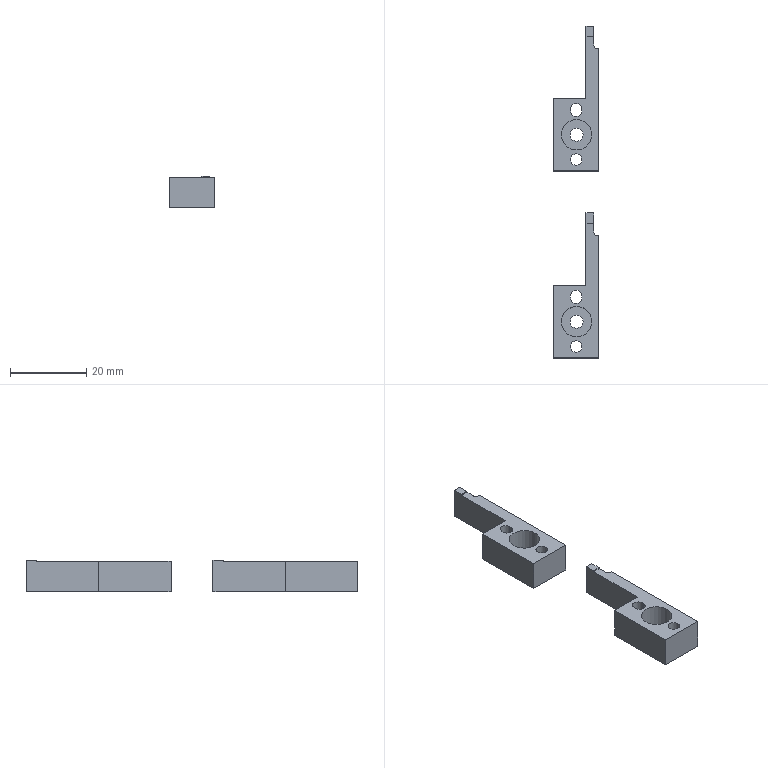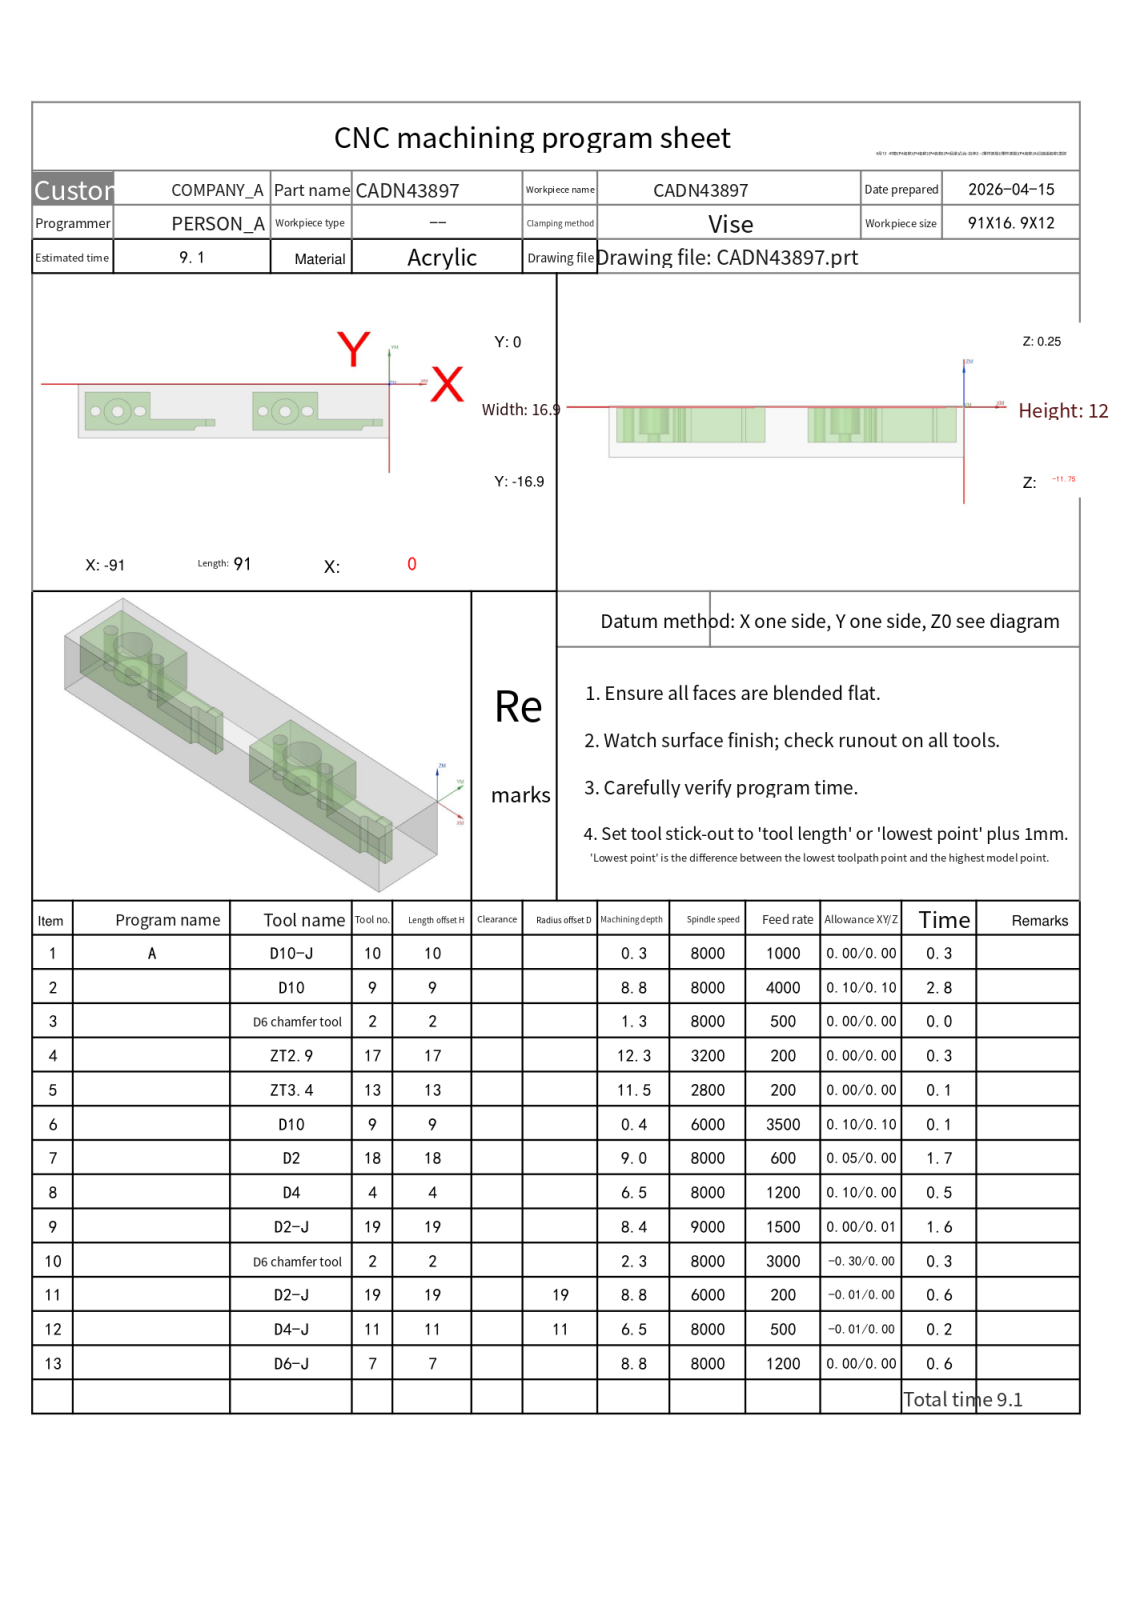NC program | NX | posted by the shop | part box 11.9 x 87 x 8.25 mm
Lines 8226 to 9110 of 9110:
N10 T02 M06
(D6 chamfer tool  D=6. R=0. H=02 ce=0.00 di=0.00)
G00 G90 G54 X-5.398 Y-9.389 M03 S8000
G43 H02 Z20.
M08
Z2.435
G01 Z-1.5 F3000.
X-5.404 Y-9.456
G03 X-5.111 Y-9.81 I.36 J0.0
G01 X-5.092 Y-9.809
X-4.989 Y-9.773
X-4.7 Y-9.74
X-3.35
X-2.
G02 X-.7 Y-11.04 I0.0 J-1.3
G01 Y-13.1
G02 X-2. Y-14.4 I-1.3 J0.0
G01 X-4.7
X-4.989 Y-14.367
X-5.092 Y-14.331
X-5.111 Y-14.33
G03 X-5.404 Y-14.684 I.067 J-.354
G01 X-5.398 Y-14.751
Z2.435
G00 Z20.
X-54.398 Y-9.389
Z2.435
G01 Z-1.5
X-54.404 Y-9.456
G03 X-54.111 Y-9.81 I.36 J0.0
G01 X-54.092 Y-9.809
X-53.989 Y-9.773
X-53.7 Y-9.74
X-51.
G02 X-49.7 Y-11.04 I0.0 J-1.3
G01 Y-12.07
Y-13.1
G02 X-51. Y-14.4 I-1.3 J0.0
G01 X-53.7
X-53.989 Y-14.367
X-54.092 Y-14.331
X-54.111 Y-14.33
G03 X-54.404 Y-14.684 I.067 J-.354
G01 X-54.398 Y-14.751
Z2.435
G00 Z6.
X-54.806 Y-14.566
Z2.512
G01 Z-1.75
X-54.78 Y-14.506
X-54.798 Y-14.441
X-54.85 Y-14.402
X-54.856 Y-14.4
X-55.7
G02 X-57. Y-15.7 I-1.3 J0.0
G01 X-60.
X-62.
X-63.
X-66.
X-67.
X-69.
X-74.
X-75.
X-77.
X-80.
X-81.
X-84.
X-86.
X-87.
X-89.
G02 X-90.3 Y-14.4 I0.0 J1.3
G01 Y-12.913
Y-11.425
Y-8.45
Y-2.5
G02 X-89. Y-1.2 I1.3 J0.0
G01 X-87.813
X-86.625
X-84.25
X-80.688
X-79.5
X-75.938
X-73.563
X-72.375
X-70.
G02 X-68.7 Y-2.5 I0.0 J-1.3
G01 Y-3.405
Y-4.31
Y-6.12
Y-9.74
X-67.763
X-66.825
X-64.95
X-62.138
X-61.2
X-58.388
X-56.513
X-55.575
X-54.843
Z2.677
G00 Z20.
X-73.125 Y-8.286
Z2.691
G01 Z-1.75
X-73.165 Y-8.436
G03 X-73.015 Y-8.696 I.3 J0.0
G01 X-73. Y-8.7
X-72.75
X-72.65 Y-8.673
X-72.577 Y-8.6
X-72.55 Y-8.5
X-72.577 Y-8.4
X-72.65 Y-8.327
X-72.75 Y-8.3
X-73.25
X-73.35 Y-8.327
X-73.423 Y-8.4
X-73.45 Y-8.5
X-73.423 Y-8.6
X-73.35 Y-8.673
X-73.25 Y-8.7
X-73.
X-72.985 Y-8.696
G03 X-72.835 Y-8.436 I-.15 J.26
G01 X-72.875 Y-8.286
Z2.691
G00 Z20.
X-5.806 Y-14.566
Z2.512
G01 Z-1.75
X-5.78 Y-14.506
X-5.798 Y-14.441
X-5.85 Y-14.402
X-5.856 Y-14.4
X-6.7
G02 X-8. Y-15.7 I-1.3 J0.0
G01 X-9.
X-10.
X-11.
X-12.
X-13.
X-14.
X-15.
X-16.
X-17.
X-18.
X-19.
X-20.
X-21.
X-22.
X-24.
X-25.
X-26.
X-27.
X-28.
X-29.
X-30.
X-31.
X-32.
X-33.
X-34.
X-35.
X-36.
X-37.
X-38.
X-40.
G02 X-41.3 Y-14.4 I0.0 J1.3
G01 Y-12.913
Y-11.425
Y-9.938
Y-8.45
Y-6.963
Y-5.475
Y-2.5
G02 X-40. Y-1.2 I1.3 J0.0
G01 X-38.813
X-37.625
X-36.438
X-35.25
X-34.063
X-32.875
X-31.688
X-30.5
X-29.313
X-28.125
X-26.938
X-25.75
X-24.563
X-23.375
X-21.
G02 X-19.7 Y-2.5 I0.0 J-1.3
G01 Y-3.405
Y-4.31
Y-5.215
Y-6.12
Y-7.025
Y-7.93
Y-9.74
X-18.763
X-17.825
X-16.888
X-15.95
X-15.013
X-14.075
X-13.138
X-12.2
X-11.263
X-10.325
X-9.388
X-8.45
X-7.513
X-6.575
X-5.843
Z2.677
G00 Z20.
X-23.875 Y-8.714
Z2.691
G01 Z-1.75
X-23.835 Y-8.564
G03 X-23.985 Y-8.304 I-.3 J0.0
G01 X-24. Y-8.3
X-24.25
X-24.35 Y-8.327
X-24.423 Y-8.4
X-24.45 Y-8.5
X-24.423 Y-8.6
X-24.35 Y-8.673
X-24.25 Y-8.7
X-23.75
X-23.65 Y-8.673
X-23.577 Y-8.6
X-23.55 Y-8.5
X-23.577 Y-8.4
X-23.65 Y-8.327
X-23.75 Y-8.3
X-24.
X-24.015 Y-8.304
G03 X-24.165 Y-8.564 I.15 J-.26
G01 X-24.125 Y-8.714
Z2.691
G00 Z20.
G00 G90 X-37. Y-8.5 M03 S8000
Z20.
G98 G81 X-37. Y-8.5 Z-2.05 R2.75 F500.
X-86.
G80
G00 Z20.
G00 G90 X-31.247 Y-5.388 M03 S8000
Z20.
Z2.25
G01 X-31.462 Y-5.44 Z2.17 F500.
X-31.828 Y-5.576 Z2.028
X-32.175 Y-5.753 Z1.886
X-32.499 Y-5.971 Z1.744
X-32.795 Y-6.225 Z1.602
X-33.059 Y-6.512 Z1.46
X-33.288 Y-6.828 Z1.318
X-33.428 Y-7.072 Z1.215
X-33.588 Y-7.428 Z1.073
X-33.705 Y-7.8 Z.931
X-33.777 Y-8.184 Z.789
X-33.803 Y-8.573 Z.647
X-33.783 Y-8.962 Z.505
X-33.717 Y-9.347 Z.363
X-33.607 Y-9.721 Z.221
X-33.453 Y-10.08 Z.079
X-33.258 Y-10.418 Z-.063
X-33.024 Y-10.73 Z-.205
X-32.756 Y-11.013 Z-.347
X-32.455 Y-11.262 Z-.489
X-32.128 Y-11.474 Z-.631
X-31.778 Y-11.646 Z-.773
X-31.41 Y-11.775 Z-.915
X-31.029 Y-11.86 Z-1.057
X-30.641 Y-11.9 Z-1.199
X-30.5 Z-1.25
G03 X-27.2 Y-8.6 I0.0 J3.3
X-30.5 Y-5.3 I-3.3 J0.0
X-33.8 Y-8.6 I0.0 J-3.3
X-30.5 Y-11.9 I3.3 J0.0
X-30.002 Y-11.862 I0.0 J3.3
G01 Z1.25
G00 Z20.
X-80.247 Y-5.388
Z2.25
G01 X-80.462 Y-5.44 Z2.17
X-80.828 Y-5.576 Z2.028
X-81.175 Y-5.753 Z1.886
X-81.499 Y-5.971 Z1.744
X-81.795 Y-6.225 Z1.602
X-82.059 Y-6.512 Z1.46
X-82.288 Y-6.828 Z1.318
X-82.428 Y-7.072 Z1.215
X-82.588 Y-7.428 Z1.073
X-82.705 Y-7.8 Z.931
X-82.777 Y-8.184 Z.789
X-82.803 Y-8.573 Z.647
X-82.783 Y-8.962 Z.505
X-82.717 Y-9.347 Z.363
X-82.607 Y-9.721 Z.221
X-82.453 Y-10.08 Z.079
X-82.258 Y-10.418 Z-.063
X-82.024 Y-10.73 Z-.205
X-81.756 Y-11.013 Z-.347
X-81.455 Y-11.262 Z-.489
X-81.128 Y-11.474 Z-.631
X-80.778 Y-11.646 Z-.773
X-80.41 Y-11.775 Z-.915
X-80.029 Y-11.86 Z-1.057
X-79.641 Y-11.9 Z-1.199
X-79.5 Z-1.25
G03 X-76.2 Y-8.6 I0.0 J3.3
X-79.5 Y-5.3 I-3.3 J0.0
X-82.8 Y-8.6 I0.0 J-3.3
X-79.5 Y-11.9 I3.3 J0.0
X-79.002 Y-11.862 I0.0 J3.3
G01 Z1.25
G00 Z20.
G91 G28 Z0.0
M05
M09
G91 G28 Z0.0
M01
N11 T19 M06
(D2-J  D=2. R=0. H=19 ce=-0.01 di=0.00)
G00 G90 G54 X-24.2 Y-8.75 M03 S6000
G43 H19 Z20.
M08
Z-1.41
G01 Z-1.91 F200.
G41 D19
Y-8.8
G03 X-24. Y-9. I.2 J0.0
G01 X-23.75
G03 X-23.25 Y-8.5 I0.0 J.5
X-23.75 Y-8. I-.5 J0.0
G01 X-24.25
G03 X-24.75 Y-8.5 I0.0 J-.5
X-24.25 Y-9. I.5 J0.0
G01 X-24.
X-23.75
G03 X-23.51 Y-8.939 I0.0 J.5
X-23.406 Y-8.763 I-.096 J.176
G01 X-23.431 Y-8.667
X-23.467 Y-8.6
G40 X-23.491 Y-8.556
Z-1.41
G00 Z.25
X-24.2 Y-8.75
Z-3.07
G01 Z-3.57
G41 D19
Y-8.8
G03 X-24. Y-9. I.2 J0.0
G01 X-23.75
G03 X-23.25 Y-8.5 I0.0 J.5
X-23.75 Y-8. I-.5 J0.0
G01 X-24.25
G03 X-24.75 Y-8.5 I0.0 J-.5
X-24.25 Y-9. I.5 J0.0
G01 X-24.
X-23.75
G03 X-23.51 Y-8.939 I0.0 J.5
X-23.406 Y-8.763 I-.096 J.176
G01 X-23.431 Y-8.667
X-23.467 Y-8.6
G40 X-23.491 Y-8.556
Z-3.07
G00 Z-1.41
X-24.2 Y-8.75
Z-4.73
G01 Z-5.23
G41 D19
Y-8.8
G03 X-24. Y-9. I.2 J0.0
G01 X-23.75
G03 X-23.25 Y-8.5 I0.0 J.5
X-23.75 Y-8. I-.5 J0.0
G01 X-24.25
G03 X-24.75 Y-8.5 I0.0 J-.5
X-24.25 Y-9. I.5 J0.0
G01 X-24.
X-23.75
G03 X-23.51 Y-8.939 I0.0 J.5
X-23.406 Y-8.763 I-.096 J.176
G01 X-23.431 Y-8.667
X-23.467 Y-8.6
G40 X-23.491 Y-8.556
Z-4.73
G00 Z-3.07
X-24.2 Y-8.75
Z-6.39
G01 Z-6.89
G41 D19
Y-8.8
G03 X-24. Y-9. I.2 J0.0
G01 X-23.75
G03 X-23.25 Y-8.5 I0.0 J.5
X-23.75 Y-8. I-.5 J0.0
G01 X-24.25
G03 X-24.75 Y-8.5 I0.0 J-.5
X-24.25 Y-9. I.5 J0.0
G01 X-24.
X-23.75
G03 X-23.51 Y-8.939 I0.0 J.5
X-23.406 Y-8.763 I-.096 J.176
G01 X-23.431 Y-8.667
X-23.467 Y-8.6
G40 X-23.491 Y-8.556
Z-6.39
G00 Z-4.73
X-24.2 Y-8.75
Z-8.05
G01 Z-8.55
G41 D19
Y-8.8
G03 X-24. Y-9. I.2 J0.0
G01 X-23.75
G03 X-23.25 Y-8.5 I0.0 J.5
X-23.75 Y-8. I-.5 J0.0
G01 X-24.25
G03 X-24.75 Y-8.5 I0.0 J-.5
X-24.25 Y-9. I.5 J0.0
G01 X-24.
X-23.75
G03 X-23.51 Y-8.939 I0.0 J.5
X-23.406 Y-8.763 I-.096 J.176
G01 X-23.431 Y-8.667
X-23.467 Y-8.6
G40 X-23.491 Y-8.556
Z-8.05
G00 Z20.
X-37.2 Y-8.674
Z-1.41
G01 Z-1.91
G41 D19
Y-8.8
G03 X-37. Y-9. I.2 J0.0
X-36.5 Y-8.5 I0.0 J.5
X-37. Y-8. I-.5 J0.0
X-37.5 Y-8.5 I0.0 J-.5
X-37. Y-9. I.5 J0.0
X-36.579 Y-8.77 I0.0 J.5
G01 X-36.548 Y-8.662
X-36.639 Y-8.494
X-36.704 Y-8.453
G40 X-36.746 Y-8.426
Z-1.41
G00 Z.25
X-37.2 Y-8.674
Z-3.07
G01 Z-3.57
G41 D19
Y-8.8
G03 X-37. Y-9. I.2 J0.0
X-36.5 Y-8.5 I0.0 J.5
X-37. Y-8. I-.5 J0.0
X-37.5 Y-8.5 I0.0 J-.5
X-37. Y-9. I.5 J0.0
X-36.579 Y-8.77 I0.0 J.5
G01 X-36.548 Y-8.662
X-36.639 Y-8.494
X-36.704 Y-8.453
G40 X-36.746 Y-8.426
Z-3.07
G00 Z-1.41
X-37.2 Y-8.674
Z-4.73
G01 Z-5.23
G41 D19
Y-8.8
G03 X-37. Y-9. I.2 J0.0
X-36.5 Y-8.5 I0.0 J.5
X-37. Y-8. I-.5 J0.0
X-37.5 Y-8.5 I0.0 J-.5
X-37. Y-9. I.5 J0.0
X-36.579 Y-8.77 I0.0 J.5
G01 X-36.548 Y-8.662
X-36.639 Y-8.494
X-36.704 Y-8.453
G40 X-36.746 Y-8.426
Z-4.73
G00 Z-3.07
X-37.2 Y-8.674
Z-6.39
G01 Z-6.89
G41 D19
Y-8.8
G03 X-37. Y-9. I.2 J0.0
X-36.5 Y-8.5 I0.0 J.5
X-37. Y-8. I-.5 J0.0
X-37.5 Y-8.5 I0.0 J-.5
X-37. Y-9. I.5 J0.0
X-36.579 Y-8.77 I0.0 J.5
G01 X-36.548 Y-8.662
X-36.639 Y-8.494
X-36.704 Y-8.453
G40 X-36.746 Y-8.426
Z-6.39
G00 Z-4.73
X-37.2 Y-8.674
Z-8.05
G01 Z-8.55
G41 D19
Y-8.8
G03 X-37. Y-9. I.2 J0.0
X-36.5 Y-8.5 I0.0 J.5
X-37. Y-8. I-.5 J0.0
X-37.5 Y-8.5 I0.0 J-.5
X-37. Y-9. I.5 J0.0
X-36.579 Y-8.77 I0.0 J.5
G01 X-36.548 Y-8.662
X-36.639 Y-8.494
X-36.704 Y-8.453
G40 X-36.746 Y-8.426
Z-8.05
G00 Z20.
X-73.2 Y-8.75
Z-1.41
G01 Z-1.91
G41 D19
Y-8.8
G03 X-73. Y-9. I.2 J0.0
G01 X-72.75
G03 X-72.25 Y-8.5 I0.0 J.5
X-72.75 Y-8. I-.5 J0.0
G01 X-73.25
G03 X-73.75 Y-8.5 I0.0 J-.5
X-73.25 Y-9. I.5 J0.0
G01 X-73.
X-72.75
G03 X-72.51 Y-8.939 I0.0 J.5
X-72.406 Y-8.763 I-.096 J.176
G01 X-72.431 Y-8.667
X-72.467 Y-8.6
G40 X-72.491 Y-8.556
Z-1.41
G00 Z.25
X-73.2 Y-8.75
Z-3.07
G01 Z-3.57
G41 D19
Y-8.8
G03 X-73. Y-9. I.2 J0.0
G01 X-72.75
G03 X-72.25 Y-8.5 I0.0 J.5
X-72.75 Y-8. I-.5 J0.0
G01 X-73.25
G03 X-73.75 Y-8.5 I0.0 J-.5
X-73.25 Y-9. I.5 J0.0
G01 X-73.
X-72.75
G03 X-72.51 Y-8.939 I0.0 J.5
X-72.406 Y-8.763 I-.096 J.176
G01 X-72.431 Y-8.667
X-72.467 Y-8.6
G40 X-72.491 Y-8.556
Z-3.07
G00 Z-1.41
X-73.2 Y-8.75
Z-4.73
G01 Z-5.23
G41 D19
Y-8.8
G03 X-73. Y-9. I.2 J0.0
G01 X-72.75
G03 X-72.25 Y-8.5 I0.0 J.5
X-72.75 Y-8. I-.5 J0.0
G01 X-73.25
G03 X-73.75 Y-8.5 I0.0 J-.5
X-73.25 Y-9. I.5 J0.0
G01 X-73.
X-72.75
G03 X-72.51 Y-8.939 I0.0 J.5
X-72.406 Y-8.763 I-.096 J.176
G01 X-72.431 Y-8.667
X-72.467 Y-8.6
G40 X-72.491 Y-8.556
Z-4.73
G00 Z-3.07
X-73.2 Y-8.75
Z-6.39
G01 Z-6.89
G41 D19
Y-8.8
G03 X-73. Y-9. I.2 J0.0
G01 X-72.75
G03 X-72.25 Y-8.5 I0.0 J.5
X-72.75 Y-8. I-.5 J0.0
G01 X-73.25
G03 X-73.75 Y-8.5 I0.0 J-.5
X-73.25 Y-9. I.5 J0.0
G01 X-73.
X-72.75
G03 X-72.51 Y-8.939 I0.0 J.5
X-72.406 Y-8.763 I-.096 J.176
G01 X-72.431 Y-8.667
X-72.467 Y-8.6
G40 X-72.491 Y-8.556
Z-6.39
G00 Z-4.73
X-73.2 Y-8.75
Z-8.05
G01 Z-8.55
G41 D19
Y-8.8
G03 X-73. Y-9. I.2 J0.0
G01 X-72.75
G03 X-72.25 Y-8.5 I0.0 J.5
X-72.75 Y-8. I-.5 J0.0
G01 X-73.25
G03 X-73.75 Y-8.5 I0.0 J-.5
X-73.25 Y-9. I.5 J0.0
G01 X-73.
X-72.75
G03 X-72.51 Y-8.939 I0.0 J.5
X-72.406 Y-8.763 I-.096 J.176
G01 X-72.431 Y-8.667
X-72.467 Y-8.6
G40 X-72.491 Y-8.556
Z-8.05
G00 Z20.
X-86.174 Y-8.3
Z-1.41
G01 Z-1.91
G41 D19
X-86.3
G03 X-86.5 Y-8.5 I0.0 J-.2
X-86. Y-9. I.5 J0.0
X-85.5 Y-8.5 I0.0 J.5
X-86. Y-8. I-.5 J0.0
X-86.5 Y-8.5 I0.0 J-.5
X-86.27 Y-8.921 I.5 J0.0
G01 X-86.162 Y-8.952
X-85.994 Y-8.861
X-85.953 Y-8.796
G40 X-85.926 Y-8.754
Z-1.41
G00 Z.25
X-86.174 Y-8.3
Z-3.07
G01 Z-3.57
G41 D19
X-86.3
G03 X-86.5 Y-8.5 I0.0 J-.2
X-86. Y-9. I.5 J0.0
X-85.5 Y-8.5 I0.0 J.5
X-86. Y-8. I-.5 J0.0
X-86.5 Y-8.5 I0.0 J-.5
X-86.27 Y-8.921 I.5 J0.0
G01 X-86.162 Y-8.952
X-85.994 Y-8.861
X-85.953 Y-8.796
G40 X-85.926 Y-8.754
Z-3.07
G00 Z-1.41
X-86.174 Y-8.3
Z-4.73
G01 Z-5.23
G41 D19
X-86.3
G03 X-86.5 Y-8.5 I0.0 J-.2
X-86. Y-9. I.5 J0.0
X-85.5 Y-8.5 I0.0 J.5
X-86. Y-8. I-.5 J0.0
X-86.5 Y-8.5 I0.0 J-.5
X-86.27 Y-8.921 I.5 J0.0
G01 X-86.162 Y-8.952
X-85.994 Y-8.861
X-85.953 Y-8.796
G40 X-85.926 Y-8.754
Z-4.73
G00 Z-3.07
X-86.174 Y-8.3
Z-6.39
G01 Z-6.89
G41 D19
X-86.3
G03 X-86.5 Y-8.5 I0.0 J-.2
X-86. Y-9. I.5 J0.0
X-85.5 Y-8.5 I0.0 J.5
X-86. Y-8. I-.5 J0.0
X-86.5 Y-8.5 I0.0 J-.5
X-86.27 Y-8.921 I.5 J0.0
G01 X-86.162 Y-8.952
X-85.994 Y-8.861
X-85.953 Y-8.796
G40 X-85.926 Y-8.754
Z-6.39
G00 Z-4.73
X-86.174 Y-8.3
Z-8.05
G01 Z-8.55
G41 D19
X-86.3
G03 X-86.5 Y-8.5 I0.0 J-.2
X-86. Y-9. I.5 J0.0
X-85.5 Y-8.5 I0.0 J.5
X-86. Y-8. I-.5 J0.0
X-86.5 Y-8.5 I0.0 J-.5
X-86.27 Y-8.921 I.5 J0.0
G01 X-86.162 Y-8.952
X-85.994 Y-8.861
X-85.953 Y-8.796
G40 X-85.926 Y-8.754
Z-8.05
G00 Z20.
G91 G28 Z0.0
M05
M09
G91 G28 Z0.0
M01
N12 T11 M06
(D4-J  D=4. R=0. H=11 ce=-0.01 di=0.00)
G00 G90 G54 X-30.5 Y-8.6 M03 S8000
G43 H11 Z20.
M08
Z.25
G41 D11
G01 X-30.696 Y-8.639 F500.
G03 X-31.495 Y-9.615 I.196 J-.976
X-30.5 Y-10.61 I.995 J0.0
X-30.5 Y-10.61 Z-4.75 I0.0 J2.01
X-28.588 Y-7.979 Z-6.25 I0.0 J2.01
X-30.5 Y-6.59 I-1.912 J-.621
X-32.51 Y-8.6 I0.0 J-2.01
X-30.5 Y-10.61 I2.01 J0.0
X-28.49 Y-8.6 I0.0 J2.01
X-28.588 Y-7.979 I-2.01 J0.0
X-29.535 Y-7.291 I-.946 J-.307
X-30.53 Y-8.286 I0.0 J-.995
G01 X-30.523 Y-8.401
G40 X-30.5 Y-8.6
G00 Z20.
X-79.5
Z.25
G41 D11
G01 X-79.696 Y-8.639
G03 X-80.495 Y-9.615 I.196 J-.976
X-79.5 Y-10.61 I.995 J0.0
X-79.5 Y-10.61 Z-4.75 I0.0 J2.01
X-77.588 Y-7.979 Z-6.25 I0.0 J2.01
X-79.5 Y-6.59 I-1.912 J-.621
X-81.51 Y-8.6 I0.0 J-2.01
X-79.5 Y-10.61 I2.01 J0.0
X-77.49 Y-8.6 I0.0 J2.01
X-77.588 Y-7.979 I-2.01 J0.0
X-78.535 Y-7.291 I-.946 J-.307
X-79.53 Y-8.286 I0.0 J-.995
G01 X-79.523 Y-8.401
G40 X-79.5 Y-8.6
G00 Z20.
G91 G28 Z0.0
M05
M09
G91 G28 Z0.0
M01
N13 T07 M06
(D6-J  D=6. R=0. H=07 ce=0.30 di=0.00)
G00 G90 G54 X-30.492 Y-20.4 M03 S6000
G43 H07 Z20.
M08
Z.25
G01 Z-.25 F1200.
Y-15.
X-40.6
Y-1.9
X-20.4
Y-10.44
X-8.
Y-15.
X-30.492
Y-10.8
X-36.4
Y-6.1
X-24.6
Y-10.44
G03 X-24.585 Y-10.8 I4.2 J0.0
G01 X-30.492
X-30.992
Y-20.4
Z.25
G00 Z20.
X-79.492
Z.25
G01 Z-.25
Y-15.
X-89.6
Y-1.9
X-69.4
Y-10.44
X-57.
Y-15.
X-79.492
Y-10.8
X-85.4
Y-6.1
X-73.6
Y-10.44
G03 X-73.585 Y-10.8 I4.2 J0.0
G01 X-79.492
X-79.992
Y-20.4
Z.25
G00 Z20.
G00 G90 X-53.3 Y-17.2 M03 S6000
Z20.
Z.255
G01 Z-.245 F1200.
G41 D07
Y-17.1
G03 X-54.3 Y-16.1 I-1. J0.0
G01 X-56.7
Y-8.34
G03 X-57.7 Y-7.34 I-1. J0.0
G01 G40 X-57.8
Z.255
G00 Z20.
X-4.3 Y-17.2
Z.255
G01 Z-.245
G41 D07
Y-17.1
G03 X-5.3 Y-16.1 I-1. J0.0
G01 X-7.7
Y-8.34
G03 X-8.7 Y-7.34 I-1. J0.0
G01 G40 X-8.8
Z.255
G00 Z20.
G00 G90 X-55.983 Y-18.473 M03 S8000
Z20.
Z-8.05
G01 Z-8.55 F1000.
G41 D07
X-56.008 Y-18.275
G03 X-57. Y-17.4 I-.992 J-.125
G01 X-89.
G02 X-92. Y-14.4 I0.0 J3.
G01 Y-2.5
G02 X-89. Y.5 I3. J0.0
G01 X-70.
G02 X-67. Y-2.5 I0.0 J-3.
G01 Y-8.04
X-51.
G02 X-48. Y-11.04 I0.0 J-3.
G01 Y-13.1
G02 X-51. Y-16.1 I-3. J0.0
G01 X-54.528
G02 X-57. Y-17.4 I-2.472 J1.7
G01 X-57.5
G03 X-58.5 Y-18.4 I0.0 J-1.
G01 G40 Y-18.6
Z-8.05
G00 Z20.
X-6.983 Y-18.473
Z-8.05
G01 Z-8.55
G41 D07
X-7.008 Y-18.275
G03 X-8. Y-17.4 I-.992 J-.125
G01 X-40.
G02 X-43. Y-14.4 I0.0 J3.
G01 Y-2.5
G02 X-40. Y.5 I3. J0.0
G01 X-21.
G02 X-18. Y-2.5 I0.0 J-3.
G01 Y-8.04
X-2.
G02 X1. Y-11.04 I0.0 J-3.
G01 Y-13.1
G02 X-2. Y-16.1 I-3. J0.0
G01 X-5.528
G02 X-8. Y-17.4 I-2.472 J1.7
G01 X-8.5
G03 X-9.5 Y-18.4 I0.0 J-1.
G01 G40 Y-18.6
Z-8.05
G00 Z20.
M05
M09
G91 G28 Z0.0
G91 G28 Y0.0
M30
%